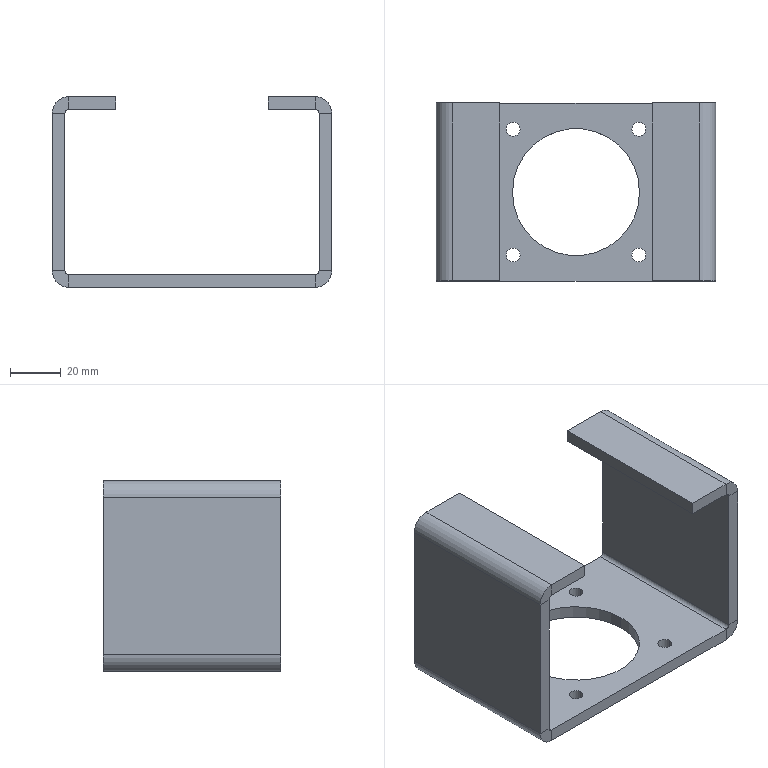Part | STEP file | Motor hanging plate SGN-5-08 | 1 solid | 48 faces | box 110 x 70 x 75 mm | volume 88804 mm3 | plane 30 | cylinder 18 | commonest cylinder face diameters 5.5 x8 3 x4 13 x4 50 x2